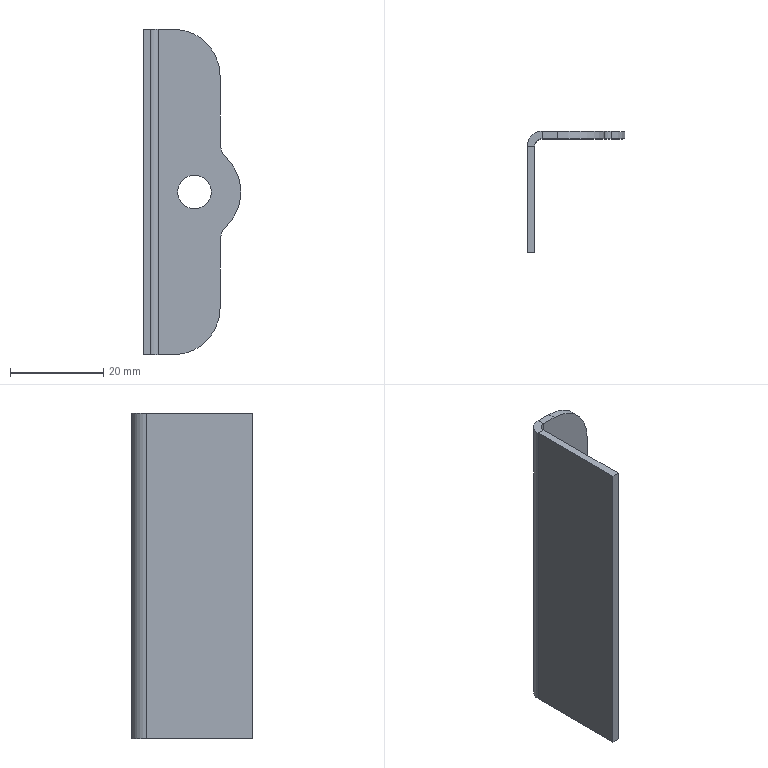Part | SolidWorks | features EdgeFlange 1, FlatPattern 1, SMBaseFlange 1, SheetMetal 1 | 1 solid | 22 faces | box 21 x 26 x 70 mm | volume 4418 mm3 | plane 13 | cylinder 9 | commonest cylinder face diameters 20 x3 7.2 x2 10 x2 3.2 x1 6.4 x1
STEP:
#1=CARTESIAN_POINT('',(2.75,-1.6,-3.6));
#2=VERTEX_POINT('',#1);
#3=CARTESIAN_POINT('',(2.75,-1.6,3.6));
#4=VERTEX_POINT('',#3);
#5=CARTESIAN_POINT('',(2.75,-1.6,0.));
#6=DIRECTION('',(0.,1.,0.));
#7=DIRECTION('',(0.,0.,1.));
#8=AXIS2_PLACEMENT_3D('',#5,#6,#7);
#9=CIRCLE('',#8,3.6);
#10=EDGE_CURVE('',#2,#4,#9,.T.);
#11=ORIENTED_EDGE('',*,*,#10,.F.);
#12=CARTESIAN_POINT('',(2.75,0.,-3.6));
#13=VERTEX_POINT('',#12);
#14=CARTESIAN_POINT('',(2.75,-1.6,-3.6));
#15=DIRECTION('',(0.,1.,0.));
#16=VECTOR('',#15,1000.);
#17=LINE('',#14,#16);
#18=EDGE_CURVE('',#2,#13,#17,.T.);
#19=ORIENTED_EDGE('',*,*,#18,.T.);
#20=CARTESIAN_POINT('',(2.75,0.,3.6));
#21=VERTEX_POINT('',#20);
#22=CARTESIAN_POINT('',(2.75,0.,0.));
#23=DIRECTION('',(0.,1.,0.));
#24=DIRECTION('',(0.,0.,1.));
#25=AXIS2_PLACEMENT_3D('',#22,#23,#24);
#26=CIRCLE('',#25,3.6);
#27=EDGE_CURVE('',#13,#21,#26,.T.);
#28=ORIENTED_EDGE('',*,*,#27,.T.);
#29=CARTESIAN_POINT('',(2.75,-1.6,3.6));
#30=DIRECTION('',(0.,1.,0.));
#31=VECTOR('',#30,1000.);
#32=LINE('',#29,#31);
#33=EDGE_CURVE('',#4,#21,#32,.T.);
#34=ORIENTED_EDGE('',*,*,#33,.F.);
#35=EDGE_LOOP('',(#11,#19,#28,#34));
#36=FACE_OUTER_BOUND('',#35,.T.);
#37=CARTESIAN_POINT('',(2.75,-1.6,0.));
#38=DIRECTION('',(0.,1.,0.));
#39=DIRECTION('',(0.,0.,1.));
#40=AXIS2_PLACEMENT_3D('',#37,#38,#39);
#41=CYLINDRICAL_SURFACE('',#40,3.6);
#42=ADVANCED_FACE('',(#36),#41,.F.);
#43=CARTESIAN_POINT('',(-1.75,-1.6,-35.));
#44=VERTEX_POINT('',#43);
#45=CARTESIAN_POINT('',(-5.05,-1.6,-35.));
#46=VERTEX_POINT('',#45);
#47=CARTESIAN_POINT('',(-8.25,-1.6,-35.));
#48=DIRECTION('',(-1.,0.,0.));
#49=VECTOR('',#48,1000.);
#50=LINE('',#47,#49);
#51=EDGE_CURVE('',#44,#46,#50,.T.);
#52=ORIENTED_EDGE('',*,*,#51,.T.);
#53=CARTESIAN_POINT('',(-5.05,0.,-35.));
#54=VERTEX_POINT('',#53);
#55=CARTESIAN_POINT('',(-5.05,-1.6,-35.));
#56=DIRECTION('',(0.,1.,0.));
#57=VECTOR('',#56,1000.);
#58=LINE('',#55,#57);
#59=EDGE_CURVE('',#46,#54,#58,.T.);
#60=ORIENTED_EDGE('',*,*,#59,.T.);
#61=CARTESIAN_POINT('',(-1.75,0.,-35.));
#62=VERTEX_POINT('',#61);
#63=CARTESIAN_POINT('',(-8.25,0.,-35.));
#64=DIRECTION('',(-1.,0.,0.));
#65=VECTOR('',#64,1000.);
#66=LINE('',#63,#65);
#67=EDGE_CURVE('',#62,#54,#66,.T.);
#68=ORIENTED_EDGE('',*,*,#67,.F.);
#69=CARTESIAN_POINT('',(-1.75,-1.6,-35.));
#70=DIRECTION('',(0.,1.,0.));
#71=VECTOR('',#70,1000.);
#72=LINE('',#69,#71);
#73=EDGE_CURVE('',#44,#62,#72,.T.);
#74=ORIENTED_EDGE('',*,*,#73,.F.);
#75=EDGE_LOOP('',(#52,#60,#68,#74));
#76=FACE_OUTER_BOUND('',#75,.T.);
#77=CARTESIAN_POINT('',(-8.25,-1.6,-35.));
#78=DIRECTION('',(0.,0.,-1.));
#79=DIRECTION('',(-1.,0.,0.));
#80=AXIS2_PLACEMENT_3D('',#77,#78,#79);
#81=PLANE('',#80);
#82=ADVANCED_FACE('',(#76),#81,.T.);
#83=CARTESIAN_POINT('',(2.75,-1.6,0.));
#84=DIRECTION('',(0.,1.,0.));
#85=DIRECTION('',(0.,0.,1.));
#86=AXIS2_PLACEMENT_3D('',#83,#84,#85);
#87=CIRCLE('',#86,3.6);
#88=EDGE_CURVE('',#4,#2,#87,.T.);
#89=ORIENTED_EDGE('',*,*,#88,.T.);
#90=ORIENTED_EDGE('',*,*,#10,.T.);
#91=EDGE_LOOP('',(#89,#90));
#92=FACE_BOUND('',#91,.T.);
#93=CARTESIAN_POINT('',(-5.05,-1.6,35.));
#94=VERTEX_POINT('',#93);
#95=CARTESIAN_POINT('',(-1.75,-1.6,35.));
#96=VERTEX_POINT('',#95);
#97=CARTESIAN_POINT('',(-8.25,-1.6,35.));
#98=DIRECTION('',(1.,0.,0.));
#99=VECTOR('',#98,1000.);
#100=LINE('',#97,#99);
#101=EDGE_CURVE('',#94,#96,#100,.T.);
#102=ORIENTED_EDGE('',*,*,#101,.F.);
#103=CARTESIAN_POINT('',(-5.05,-1.6,-35.));
#104=DIRECTION('',(0.,0.,1.));
#105=VECTOR('',#104,1000.);
#106=LINE('',#103,#105);
#107=EDGE_CURVE('',#46,#94,#106,.T.);
#108=ORIENTED_EDGE('',*,*,#107,.F.);
#109=ORIENTED_EDGE('',*,*,#51,.F.);
#110=CARTESIAN_POINT('',(8.25,-1.6,-25.));
#111=VERTEX_POINT('',#110);
#112=CARTESIAN_POINT('',(-1.75,-1.6,-25.));
#113=DIRECTION('',(0.,1.,0.));
#114=DIRECTION('',(0.,0.,1.));
#115=AXIS2_PLACEMENT_3D('',#112,#113,#114);
#116=CIRCLE('',#115,10.);
#117=EDGE_CURVE('',#111,#44,#116,.T.);
#118=ORIENTED_EDGE('',*,*,#117,.F.);
#119=CARTESIAN_POINT('',(8.25,-1.6,-10.712));
#120=VERTEX_POINT('',#119);
#121=CARTESIAN_POINT('',(8.25,-1.6,-25.));
#122=DIRECTION('',(0.,0.,-1.));
#123=VECTOR('',#122,1000.);
#124=LINE('',#121,#123);
#125=EDGE_CURVE('',#120,#111,#124,.T.);
#126=ORIENTED_EDGE('',*,*,#125,.F.);
#127=CARTESIAN_POINT('',(9.75,-1.6,-7.141));
#128=VERTEX_POINT('',#127);
#129=CARTESIAN_POINT('',(13.25,-1.6,-10.712));
#130=DIRECTION('',(0.,-1.,0.));
#131=DIRECTION('',(0.,0.,1.));
#132=AXIS2_PLACEMENT_3D('',#129,#130,#131);
#133=CIRCLE('',#132,5.);
#134=EDGE_CURVE('',#128,#120,#133,.T.);
#135=ORIENTED_EDGE('',*,*,#134,.F.);
#136=CARTESIAN_POINT('',(9.75,-1.6,7.141));
#137=VERTEX_POINT('',#136);
#138=CARTESIAN_POINT('',(2.75,-1.6,0.));
#139=DIRECTION('',(0.,1.,0.));
#140=DIRECTION('',(0.,0.,1.));
#141=AXIS2_PLACEMENT_3D('',#138,#139,#140);
#142=CIRCLE('',#141,10.);
#143=EDGE_CURVE('',#137,#128,#142,.T.);
#144=ORIENTED_EDGE('',*,*,#143,.F.);
#145=CARTESIAN_POINT('',(8.25,-1.6,10.712));
#146=VERTEX_POINT('',#145);
#147=CARTESIAN_POINT('',(13.25,-1.6,10.712));
#148=DIRECTION('',(0.,-1.,0.));
#149=DIRECTION('',(0.,0.,1.));
#150=AXIS2_PLACEMENT_3D('',#147,#148,#149);
#151=CIRCLE('',#150,5.);
#152=EDGE_CURVE('',#146,#137,#151,.T.);
#153=ORIENTED_EDGE('',*,*,#152,.F.);
#154=CARTESIAN_POINT('',(8.25,-1.6,25.));
#155=VERTEX_POINT('',#154);
#156=CARTESIAN_POINT('',(8.25,-1.6,10.712));
#157=DIRECTION('',(0.,0.,-1.));
#158=VECTOR('',#157,1000.);
#159=LINE('',#156,#158);
#160=EDGE_CURVE('',#155,#146,#159,.T.);
#161=ORIENTED_EDGE('',*,*,#160,.F.);
#162=CARTESIAN_POINT('',(-1.75,-1.6,25.));
#163=DIRECTION('',(0.,1.,0.));
#164=DIRECTION('',(0.,0.,-1.));
#165=AXIS2_PLACEMENT_3D('',#162,#163,#164);
#166=CIRCLE('',#165,10.);
#167=EDGE_CURVE('',#96,#155,#166,.T.);
#168=ORIENTED_EDGE('',*,*,#167,.F.);
#169=EDGE_LOOP('',(#102,#108,#109,#118,#126,#135,#144,#153,#161,#168));
#170=FACE_OUTER_BOUND('',#169,.T.);
#171=CARTESIAN_POINT('',(-1.75,-1.6,25.));
#172=DIRECTION('',(0.,-1.,0.));
#173=DIRECTION('',(0.,0.,-1.));
#174=AXIS2_PLACEMENT_3D('',#171,#172,#173);
#175=PLANE('',#174);
#176=ADVANCED_FACE('',(#92,#170),#175,.T.);
#177=CARTESIAN_POINT('',(2.75,0.,0.));
#178=DIRECTION('',(0.,1.,0.));
#179=DIRECTION('',(0.,0.,1.));
#180=AXIS2_PLACEMENT_3D('',#177,#178,#179);
#181=CIRCLE('',#180,3.6);
#182=EDGE_CURVE('',#21,#13,#181,.T.);
#183=ORIENTED_EDGE('',*,*,#182,.F.);
#184=ORIENTED_EDGE('',*,*,#27,.F.);
#185=EDGE_LOOP('',(#183,#184));
#186=FACE_BOUND('',#185,.T.);
#187=CARTESIAN_POINT('',(-5.05,0.,35.));
#188=VERTEX_POINT('',#187);
#189=CARTESIAN_POINT('',(-5.05,0.,-35.));
#190=DIRECTION('',(0.,0.,1.));
#191=VECTOR('',#190,1000.);
#192=LINE('',#189,#191);
#193=EDGE_CURVE('',#54,#188,#192,.T.);
#194=ORIENTED_EDGE('',*,*,#193,.T.);
#195=CARTESIAN_POINT('',(-1.75,0.,35.));
#196=VERTEX_POINT('',#195);
#197=CARTESIAN_POINT('',(-8.25,0.,35.));
#198=DIRECTION('',(1.,0.,0.));
#199=VECTOR('',#198,1000.);
#200=LINE('',#197,#199);
#201=EDGE_CURVE('',#188,#196,#200,.T.);
#202=ORIENTED_EDGE('',*,*,#201,.T.);
#203=CARTESIAN_POINT('',(8.25,0.,25.));
#204=VERTEX_POINT('',#203);
#205=CARTESIAN_POINT('',(-1.75,0.,25.));
#206=DIRECTION('',(0.,1.,0.));
#207=DIRECTION('',(0.,0.,-1.));
#208=AXIS2_PLACEMENT_3D('',#205,#206,#207);
#209=CIRCLE('',#208,10.);
#210=EDGE_CURVE('',#196,#204,#209,.T.);
#211=ORIENTED_EDGE('',*,*,#210,.T.);
#212=CARTESIAN_POINT('',(8.25,0.,10.712));
#213=VERTEX_POINT('',#212);
#214=CARTESIAN_POINT('',(8.25,0.,10.712));
#215=DIRECTION('',(0.,0.,-1.));
#216=VECTOR('',#215,1000.);
#217=LINE('',#214,#216);
#218=EDGE_CURVE('',#204,#213,#217,.T.);
#219=ORIENTED_EDGE('',*,*,#218,.T.);
#220=CARTESIAN_POINT('',(9.75,0.,7.141));
#221=VERTEX_POINT('',#220);
#222=CARTESIAN_POINT('',(13.25,0.,10.712));
#223=DIRECTION('',(0.,-1.,0.));
#224=DIRECTION('',(0.,0.,1.));
#225=AXIS2_PLACEMENT_3D('',#222,#223,#224);
#226=CIRCLE('',#225,5.);
#227=EDGE_CURVE('',#213,#221,#226,.T.);
#228=ORIENTED_EDGE('',*,*,#227,.T.);
#229=CARTESIAN_POINT('',(9.75,0.,-7.141));
#230=VERTEX_POINT('',#229);
#231=CARTESIAN_POINT('',(2.75,0.,0.));
#232=DIRECTION('',(0.,1.,0.));
#233=DIRECTION('',(0.,0.,1.));
#234=AXIS2_PLACEMENT_3D('',#231,#232,#233);
#235=CIRCLE('',#234,10.);
#236=EDGE_CURVE('',#221,#230,#235,.T.);
#237=ORIENTED_EDGE('',*,*,#236,.T.);
#238=CARTESIAN_POINT('',(8.25,0.,-10.712));
#239=VERTEX_POINT('',#238);
#240=CARTESIAN_POINT('',(13.25,0.,-10.712));
#241=DIRECTION('',(0.,-1.,0.));
#242=DIRECTION('',(0.,0.,1.));
#243=AXIS2_PLACEMENT_3D('',#240,#241,#242);
#244=CIRCLE('',#243,5.);
#245=EDGE_CURVE('',#230,#239,#244,.T.);
#246=ORIENTED_EDGE('',*,*,#245,.T.);
#247=CARTESIAN_POINT('',(8.25,0.,-25.));
#248=VERTEX_POINT('',#247);
#249=CARTESIAN_POINT('',(8.25,0.,-25.));
#250=DIRECTION('',(0.,0.,-1.));
#251=VECTOR('',#250,1000.);
#252=LINE('',#249,#251);
#253=EDGE_CURVE('',#239,#248,#252,.T.);
#254=ORIENTED_EDGE('',*,*,#253,.T.);
#255=CARTESIAN_POINT('',(-1.75,0.,-25.));
#256=DIRECTION('',(0.,1.,0.));
#257=DIRECTION('',(0.,0.,1.));
#258=AXIS2_PLACEMENT_3D('',#255,#256,#257);
#259=CIRCLE('',#258,10.);
#260=EDGE_CURVE('',#248,#62,#259,.T.);
#261=ORIENTED_EDGE('',*,*,#260,.T.);
#262=ORIENTED_EDGE('',*,*,#67,.T.);
#263=EDGE_LOOP('',(#194,#202,#211,#219,#228,#237,#246,#254,#261,#262));
#264=FACE_OUTER_BOUND('',#263,.T.);
#265=CARTESIAN_POINT('',(-1.75,0.,25.));
#266=DIRECTION('',(0.,-1.,0.));
#267=DIRECTION('',(0.,0.,-1.));
#268=AXIS2_PLACEMENT_3D('',#265,#266,#267);
#269=PLANE('',#268);
#270=ADVANCED_FACE('',(#186,#264),#269,.F.);
#271=ORIENTED_EDGE('',*,*,#260,.F.);
#272=CARTESIAN_POINT('',(8.25,-1.6,-25.));
#273=DIRECTION('',(0.,1.,0.));
#274=VECTOR('',#273,1000.);
#275=LINE('',#272,#274);
#276=EDGE_CURVE('',#111,#248,#275,.T.);
#277=ORIENTED_EDGE('',*,*,#276,.F.);
#278=ORIENTED_EDGE('',*,*,#117,.T.);
#279=ORIENTED_EDGE('',*,*,#73,.T.);
#280=EDGE_LOOP('',(#271,#277,#278,#279));
#281=FACE_OUTER_BOUND('',#280,.T.);
#282=CARTESIAN_POINT('',(-1.75,-1.6,-25.));
#283=DIRECTION('',(0.,1.,0.));
#284=DIRECTION('',(0.,0.,1.));
#285=AXIS2_PLACEMENT_3D('',#282,#283,#284);
#286=CYLINDRICAL_SURFACE('',#285,10.);
#287=ADVANCED_FACE('',(#281),#286,.T.);
#288=ORIENTED_EDGE('',*,*,#253,.F.);
#289=CARTESIAN_POINT('',(8.25,-1.6,-10.712));
#290=DIRECTION('',(0.,1.,0.));
#291=VECTOR('',#290,1000.);
#292=LINE('',#289,#291);
#293=EDGE_CURVE('',#120,#239,#292,.T.);
#294=ORIENTED_EDGE('',*,*,#293,.F.);
#295=ORIENTED_EDGE('',*,*,#125,.T.);
#296=ORIENTED_EDGE('',*,*,#276,.T.);
#297=EDGE_LOOP('',(#288,#294,#295,#296));
#298=FACE_OUTER_BOUND('',#297,.T.);
#299=CARTESIAN_POINT('',(8.25,-1.6,-25.));
#300=DIRECTION('',(1.,0.,0.));
#301=DIRECTION('',(0.,0.,-1.));
#302=AXIS2_PLACEMENT_3D('',#299,#300,#301);
#303=PLANE('',#302);
#304=ADVANCED_FACE('',(#298),#303,.T.);
#305=ORIENTED_EDGE('',*,*,#245,.F.);
#306=CARTESIAN_POINT('',(9.75,-1.6,-7.141));
#307=DIRECTION('',(0.,1.,0.));
#308=VECTOR('',#307,1000.);
#309=LINE('',#306,#308);
#310=EDGE_CURVE('',#128,#230,#309,.T.);
#311=ORIENTED_EDGE('',*,*,#310,.F.);
#312=ORIENTED_EDGE('',*,*,#134,.T.);
#313=ORIENTED_EDGE('',*,*,#293,.T.);
#314=EDGE_LOOP('',(#305,#311,#312,#313));
#315=FACE_OUTER_BOUND('',#314,.T.);
#316=CARTESIAN_POINT('',(13.25,-1.6,-10.712));
#317=DIRECTION('',(0.,1.,0.));
#318=DIRECTION('',(0.,0.,1.));
#319=AXIS2_PLACEMENT_3D('',#316,#317,#318);
#320=CYLINDRICAL_SURFACE('',#319,5.);
#321=ADVANCED_FACE('',(#315),#320,.F.);
#322=ORIENTED_EDGE('',*,*,#236,.F.);
#323=CARTESIAN_POINT('',(9.75,-1.6,7.141));
#324=DIRECTION('',(0.,1.,0.));
#325=VECTOR('',#324,1000.);
#326=LINE('',#323,#325);
#327=EDGE_CURVE('',#137,#221,#326,.T.);
#328=ORIENTED_EDGE('',*,*,#327,.F.);
#329=ORIENTED_EDGE('',*,*,#143,.T.);
#330=ORIENTED_EDGE('',*,*,#310,.T.);
#331=EDGE_LOOP('',(#322,#328,#329,#330));
#332=FACE_OUTER_BOUND('',#331,.T.);
#333=CARTESIAN_POINT('',(2.75,-1.6,0.));
#334=DIRECTION('',(0.,1.,0.));
#335=DIRECTION('',(0.,0.,1.));
#336=AXIS2_PLACEMENT_3D('',#333,#334,#335);
#337=CYLINDRICAL_SURFACE('',#336,10.);
#338=ADVANCED_FACE('',(#332),#337,.T.);
#339=ORIENTED_EDGE('',*,*,#227,.F.);
#340=CARTESIAN_POINT('',(8.25,-1.6,10.712));
#341=DIRECTION('',(0.,1.,0.));
#342=VECTOR('',#341,1000.);
#343=LINE('',#340,#342);
#344=EDGE_CURVE('',#146,#213,#343,.T.);
#345=ORIENTED_EDGE('',*,*,#344,.F.);
#346=ORIENTED_EDGE('',*,*,#152,.T.);
#347=ORIENTED_EDGE('',*,*,#327,.T.);
#348=EDGE_LOOP('',(#339,#345,#346,#347));
#349=FACE_OUTER_BOUND('',#348,.T.);
#350=CARTESIAN_POINT('',(13.25,-1.6,10.712));
#351=DIRECTION('',(0.,1.,0.));
#352=DIRECTION('',(0.,0.,1.));
#353=AXIS2_PLACEMENT_3D('',#350,#351,#352);
#354=CYLINDRICAL_SURFACE('',#353,5.);
#355=ADVANCED_FACE('',(#349),#354,.F.);
#356=ORIENTED_EDGE('',*,*,#218,.F.);
#357=CARTESIAN_POINT('',(8.25,-1.6,25.));
#358=DIRECTION('',(0.,1.,0.));
#359=VECTOR('',#358,1000.);
#360=LINE('',#357,#359);
#361=EDGE_CURVE('',#155,#204,#360,.T.);
#362=ORIENTED_EDGE('',*,*,#361,.F.);
#363=ORIENTED_EDGE('',*,*,#160,.T.);
#364=ORIENTED_EDGE('',*,*,#344,.T.);
#365=EDGE_LOOP('',(#356,#362,#363,#364));
#366=FACE_OUTER_BOUND('',#365,.T.);
#367=CARTESIAN_POINT('',(8.25,-1.6,10.712));
#368=DIRECTION('',(1.,0.,0.));
#369=DIRECTION('',(0.,0.,-1.));
#370=AXIS2_PLACEMENT_3D('',#367,#368,#369);
#371=PLANE('',#370);
#372=ADVANCED_FACE('',(#366),#371,.T.);
#373=ORIENTED_EDGE('',*,*,#210,.F.);
#374=CARTESIAN_POINT('',(-1.75,-1.6,35.));
#375=DIRECTION('',(0.,1.,0.));
#376=VECTOR('',#375,1000.);
#377=LINE('',#374,#376);
#378=EDGE_CURVE('',#96,#196,#377,.T.);
#379=ORIENTED_EDGE('',*,*,#378,.F.);
#380=ORIENTED_EDGE('',*,*,#167,.T.);
#381=ORIENTED_EDGE('',*,*,#361,.T.);
#382=EDGE_LOOP('',(#373,#379,#380,#381));
#383=FACE_OUTER_BOUND('',#382,.T.);
#384=CARTESIAN_POINT('',(-1.75,-1.6,25.));
#385=DIRECTION('',(0.,1.,0.));
#386=DIRECTION('',(0.,0.,1.));
#387=AXIS2_PLACEMENT_3D('',#384,#385,#386);
#388=CYLINDRICAL_SURFACE('',#387,10.);
#389=ADVANCED_FACE('',(#383),#388,.T.);
#390=CARTESIAN_POINT('',(-5.05,-1.6,35.));
#391=DIRECTION('',(0.,1.,0.));
#392=VECTOR('',#391,1000.);
#393=LINE('',#390,#392);
#394=EDGE_CURVE('',#94,#188,#393,.T.);
#395=ORIENTED_EDGE('',*,*,#394,.F.);
#396=ORIENTED_EDGE('',*,*,#101,.T.);
#397=ORIENTED_EDGE('',*,*,#378,.T.);
#398=ORIENTED_EDGE('',*,*,#201,.F.);
#399=EDGE_LOOP('',(#395,#396,#397,#398));
#400=FACE_OUTER_BOUND('',#399,.T.);
#401=CARTESIAN_POINT('',(-8.25,-1.6,35.));
#402=DIRECTION('',(0.,0.,1.));
#403=DIRECTION('',(1.,0.,0.));
#404=AXIS2_PLACEMENT_3D('',#401,#402,#403);
#405=PLANE('',#404);
#406=ADVANCED_FACE('',(#400),#405,.T.);
#407=ORIENTED_EDGE('',*,*,#18,.F.);
#408=ORIENTED_EDGE('',*,*,#88,.F.);
#409=ORIENTED_EDGE('',*,*,#33,.T.);
#410=ORIENTED_EDGE('',*,*,#182,.T.);
#411=EDGE_LOOP('',(#407,#408,#409,#410));
#412=FACE_OUTER_BOUND('',#411,.T.);
#413=CARTESIAN_POINT('',(2.75,-1.6,0.));
#414=DIRECTION('',(0.,1.,0.));
#415=DIRECTION('',(0.,0.,1.));
#416=AXIS2_PLACEMENT_3D('',#413,#414,#415);
#417=CYLINDRICAL_SURFACE('',#416,3.6);
#418=ADVANCED_FACE('',(#412),#417,.F.);
#419=CARTESIAN_POINT('',(-6.65,-3.2,35.));
#420=VERTEX_POINT('',#419);
#421=CARTESIAN_POINT('',(-8.25,-3.2,35.));
#422=VERTEX_POINT('',#421);
#423=CARTESIAN_POINT('',(-8.25,-3.2,35.));
#424=DIRECTION('',(-1.,0.,0.));
#425=VECTOR('',#424,1000.);
#426=LINE('',#423,#425);
#427=EDGE_CURVE('',#420,#422,#426,.T.);
#428=ORIENTED_EDGE('',*,*,#427,.F.);
#429=CARTESIAN_POINT('',(-5.05,-3.2,35.));
#430=DIRECTION('',(0.,0.,1.));
#431=DIRECTION('',(-1.,0.,0.));
#432=AXIS2_PLACEMENT_3D('',#429,#430,#431);
#433=CIRCLE('',#432,1.6);
#434=EDGE_CURVE('',#94,#420,#433,.T.);
#435=ORIENTED_EDGE('',*,*,#434,.F.);
#436=ORIENTED_EDGE('',*,*,#394,.T.);
#437=CARTESIAN_POINT('',(-5.05,-3.2,35.));
#438=DIRECTION('',(0.,0.,1.));
#439=DIRECTION('',(-1.,0.,0.));
#440=AXIS2_PLACEMENT_3D('',#437,#438,#439);
#441=CIRCLE('',#440,3.2);
#442=EDGE_CURVE('',#188,#422,#441,.T.);
#443=ORIENTED_EDGE('',*,*,#442,.T.);
#444=EDGE_LOOP('',(#428,#435,#436,#443));
#445=FACE_OUTER_BOUND('',#444,.T.);
#446=CARTESIAN_POINT('',(-5.05,-3.2,35.));
#447=DIRECTION('',(0.,0.,1.));
#448=DIRECTION('',(1.,0.,0.));
#449=AXIS2_PLACEMENT_3D('',#446,#447,#448);
#450=PLANE('',#449);
#451=ADVANCED_FACE('',(#445),#450,.T.);
#452=CARTESIAN_POINT('',(-6.65,-3.2,-35.));
#453=VERTEX_POINT('',#452);
#454=CARTESIAN_POINT('',(-5.05,-3.2,-35.));
#455=DIRECTION('',(0.,0.,-1.));
#456=DIRECTION('',(-1.,0.,0.));
#457=AXIS2_PLACEMENT_3D('',#454,#455,#456);
#458=CIRCLE('',#457,1.6);
#459=EDGE_CURVE('',#453,#46,#458,.T.);
#460=ORIENTED_EDGE('',*,*,#459,.F.);
#461=CARTESIAN_POINT('',(-8.25,-3.2,-35.));
#462=VERTEX_POINT('',#461);
#463=CARTESIAN_POINT('',(-6.65,-3.2,-35.));
#464=DIRECTION('',(-1.,0.,0.));
#465=VECTOR('',#464,1000.);
#466=LINE('',#463,#465);
#467=EDGE_CURVE('',#453,#462,#466,.T.);
#468=ORIENTED_EDGE('',*,*,#467,.T.);
#469=CARTESIAN_POINT('',(-5.05,-3.2,-35.));
#470=DIRECTION('',(0.,0.,-1.));
#471=DIRECTION('',(-1.,0.,0.));
#472=AXIS2_PLACEMENT_3D('',#469,#470,#471);
#473=CIRCLE('',#472,3.2);
#474=EDGE_CURVE('',#462,#54,#473,.T.);
#475=ORIENTED_EDGE('',*,*,#474,.T.);
#476=ORIENTED_EDGE('',*,*,#59,.F.);
#477=EDGE_LOOP('',(#460,#468,#475,#476));
#478=FACE_OUTER_BOUND('',#477,.T.);
#479=CARTESIAN_POINT('',(-5.05,-3.2,-35.));
#480=DIRECTION('',(0.,0.,1.));
#481=DIRECTION('',(1.,0.,0.));
#482=AXIS2_PLACEMENT_3D('',#479,#480,#481);
#483=PLANE('',#482);
#484=ADVANCED_FACE('',(#478),#483,.F.);
#485=ORIENTED_EDGE('',*,*,#193,.F.);
#486=ORIENTED_EDGE('',*,*,#474,.F.);
#487=CARTESIAN_POINT('',(-8.25,-3.2,35.));
#488=DIRECTION('',(0.,0.,1.));
#489=VECTOR('',#488,1000.);
#490=LINE('',#487,#489);
#491=EDGE_CURVE('',#462,#422,#490,.T.);
#492=ORIENTED_EDGE('',*,*,#491,.T.);
#493=ORIENTED_EDGE('',*,*,#442,.F.);
#494=EDGE_LOOP('',(#485,#486,#492,#493));
#495=FACE_OUTER_BOUND('',#494,.T.);
#496=CARTESIAN_POINT('',(-5.05,-3.2,-35.));
#497=DIRECTION('',(0.,0.,-1.));
#498=DIRECTION('',(-1.,0.,0.));
#499=AXIS2_PLACEMENT_3D('',#496,#497,#498);
#500=CYLINDRICAL_SURFACE('',#499,3.2);
#501=ADVANCED_FACE('',(#495),#500,.T.);
#502=ORIENTED_EDGE('',*,*,#107,.T.);
#503=ORIENTED_EDGE('',*,*,#434,.T.);
#504=CARTESIAN_POINT('',(-6.65,-3.2,35.));
#505=DIRECTION('',(0.,0.,-1.));
#506=VECTOR('',#505,1000.);
#507=LINE('',#504,#506);
#508=EDGE_CURVE('',#420,#453,#507,.T.);
#509=ORIENTED_EDGE('',*,*,#508,.T.);
#510=ORIENTED_EDGE('',*,*,#459,.T.);
#511=EDGE_LOOP('',(#502,#503,#509,#510));
#512=FACE_OUTER_BOUND('',#511,.T.);
#513=CARTESIAN_POINT('',(-5.05,-3.2,-35.));
#514=DIRECTION('',(0.,0.,-1.));
#515=DIRECTION('',(-1.,0.,0.));
#516=AXIS2_PLACEMENT_3D('',#513,#514,#515);
#517=CYLINDRICAL_SURFACE('',#516,1.6);
#518=ADVANCED_FACE('',(#512),#517,.F.);
#519=ORIENTED_EDGE('',*,*,#467,.F.);
#520=CARTESIAN_POINT('',(-6.65,-26.,-35.));
#521=VERTEX_POINT('',#520);
#522=CARTESIAN_POINT('',(-6.65,-26.,-35.));
#523=DIRECTION('',(0.,-1.,0.));
#524=VECTOR('',#523,1000.);
#525=LINE('',#522,#524);
#526=EDGE_CURVE('',#453,#521,#525,.T.);
#527=ORIENTED_EDGE('',*,*,#526,.T.);
#528=CARTESIAN_POINT('',(-8.25,-26.,-35.));
#529=VERTEX_POINT('',#528);
#530=CARTESIAN_POINT('',(-8.25,-26.,-35.));
#531=DIRECTION('',(1.,0.,0.));
#532=VECTOR('',#531,1000.);
#533=LINE('',#530,#532);
#534=EDGE_CURVE('',#529,#521,#533,.T.);
#535=ORIENTED_EDGE('',*,*,#534,.F.);
#536=CARTESIAN_POINT('',(-8.25,0.,-35.));
#537=DIRECTION('',(0.,-1.,0.));
#538=VECTOR('',#537,1000.);
#539=LINE('',#536,#538);
#540=EDGE_CURVE('',#462,#529,#539,.T.);
#541=ORIENTED_EDGE('',*,*,#540,.F.);
#542=EDGE_LOOP('',(#519,#527,#535,#541));
#543=FACE_OUTER_BOUND('',#542,.T.);
#544=CARTESIAN_POINT('',(-8.25,-26.,-35.));
#545=DIRECTION('',(0.,0.,1.));
#546=DIRECTION('',(1.,0.,0.));
#547=AXIS2_PLACEMENT_3D('',#544,#545,#546);
#548=PLANE('',#547);
#549=ADVANCED_FACE('',(#543),#548,.F.);
#550=ORIENTED_EDGE('',*,*,#427,.T.);
#551=CARTESIAN_POINT('',(-8.25,-26.,35.));
#552=VERTEX_POINT('',#551);
#553=CARTESIAN_POINT('',(-8.25,0.,35.));
#554=DIRECTION('',(0.,1.,0.));
#555=VECTOR('',#554,1000.);
#556=LINE('',#553,#555);
#557=EDGE_CURVE('',#552,#422,#556,.T.);
#558=ORIENTED_EDGE('',*,*,#557,.F.);
#559=CARTESIAN_POINT('',(-6.65,-26.,35.));
#560=VERTEX_POINT('',#559);
#561=CARTESIAN_POINT('',(-8.25,-26.,35.));
#562=DIRECTION('',(1.,0.,0.));
#563=VECTOR('',#562,1000.);
#564=LINE('',#561,#563);
#565=EDGE_CURVE('',#552,#560,#564,.T.);
#566=ORIENTED_EDGE('',*,*,#565,.T.);
#567=CARTESIAN_POINT('',(-6.65,-1.6,35.));
#568=DIRECTION('',(0.,1.,0.));
#569=VECTOR('',#568,1000.);
#570=LINE('',#567,#569);
#571=EDGE_CURVE('',#560,#420,#570,.T.);
#572=ORIENTED_EDGE('',*,*,#571,.T.);
#573=EDGE_LOOP('',(#550,#558,#566,#572));
#574=FACE_OUTER_BOUND('',#573,.T.);
#575=CARTESIAN_POINT('',(-8.25,-1.6,35.));
#576=DIRECTION('',(0.,0.,-1.));
#577=DIRECTION('',(-1.,0.,0.));
#578=AXIS2_PLACEMENT_3D('',#575,#576,#577);
#579=PLANE('',#578);
#580=ADVANCED_FACE('',(#574),#579,.F.);
#581=ORIENTED_EDGE('',*,*,#491,.F.);
#582=ORIENTED_EDGE('',*,*,#540,.T.);
#583=CARTESIAN_POINT('',(-8.25,-26.,0.));
#584=DIRECTION('',(0.,0.,1.));
#585=VECTOR('',#584,1000.);
#586=LINE('',#583,#585);
#587=EDGE_CURVE('',#529,#552,#586,.T.);
#588=ORIENTED_EDGE('',*,*,#587,.T.);
#589=ORIENTED_EDGE('',*,*,#557,.T.);
#590=EDGE_LOOP('',(#581,#582,#588,#589));
#591=FACE_OUTER_BOUND('',#590,.T.);
#592=CARTESIAN_POINT('',(-8.25,0.,0.));
#593=DIRECTION('',(1.,0.,0.));
#594=DIRECTION('',(0.,1.,0.));
#595=AXIS2_PLACEMENT_3D('',#592,#593,#594);
#596=PLANE('',#595);
#597=ADVANCED_FACE('',(#591),#596,.F.);
#598=ORIENTED_EDGE('',*,*,#526,.F.);
#599=ORIENTED_EDGE('',*,*,#508,.F.);
#600=ORIENTED_EDGE('',*,*,#571,.F.);
#601=CARTESIAN_POINT('',(-6.65,-26.,35.));
#602=DIRECTION('',(0.,0.,1.));
#603=VECTOR('',#602,1000.);
#604=LINE('',#601,#603);
#605=EDGE_CURVE('',#521,#560,#604,.T.);
#606=ORIENTED_EDGE('',*,*,#605,.F.);
#607=EDGE_LOOP('',(#598,#599,#600,#606));
#608=FACE_OUTER_BOUND('',#607,.T.);
#609=CARTESIAN_POINT('',(-6.65,0.,0.));
#610=DIRECTION('',(1.,0.,0.));
#611=DIRECTION('',(0.,1.,0.));
#612=AXIS2_PLACEMENT_3D('',#609,#610,#611);
#613=PLANE('',#612);
#614=ADVANCED_FACE('',(#608),#613,.T.);
#615=ORIENTED_EDGE('',*,*,#605,.T.);
#616=ORIENTED_EDGE('',*,*,#565,.F.);
#617=ORIENTED_EDGE('',*,*,#587,.F.);
#618=ORIENTED_EDGE('',*,*,#534,.T.);
#619=EDGE_LOOP('',(#615,#616,#617,#618));
#620=FACE_OUTER_BOUND('',#619,.T.);
#621=CARTESIAN_POINT('',(-8.25,-26.,35.));
#622=DIRECTION('',(0.,1.,0.));
#623=DIRECTION('',(-1.,0.,0.));
#624=AXIS2_PLACEMENT_3D('',#621,#622,#623);
#625=PLANE('',#624);
#626=ADVANCED_FACE('',(#620),#625,.F.);
#627=CLOSED_SHELL('',(#42,#82,#176,#270,#287,#304,#321,#338,#355,#372,#389,#406,#418,#451,#484,#501,#518,#549,#580,#597,#614,#626));
#628=MANIFOLD_SOLID_BREP('',#627);
#629=CARTESIAN_POINT('',(0.,0.,0.));
#630=DIRECTION('',(0.,0.,1.));
#631=DIRECTION('',(1.,0.,0.));
#632=AXIS2_PLACEMENT_3D('',#629,#630,#631);
#633=(LENGTH_UNIT()NAMED_UNIT(*)SI_UNIT(.MILLI.,.METRE.));
#634=UNCERTAINTY_MEASURE_WITH_UNIT(LENGTH_MEASURE(0.00001),#633,'','');
#635=(NAMED_UNIT(*)PLANE_ANGLE_UNIT()SI_UNIT($,.RADIAN.));
#636=(NAMED_UNIT(*)SI_UNIT($,.STERADIAN.)SOLID_ANGLE_UNIT());
#637=(GEOMETRIC_REPRESENTATION_CONTEXT(3)GLOBAL_UNCERTAINTY_ASSIGNED_CONTEXT((#634))GLOBAL_UNIT_ASSIGNED_CONTEXT((#633,#635,#636))REPRESENTATION_CONTEXT('',''));
#638=ADVANCED_BREP_SHAPE_REPRESENTATION('',(#628,#632),#637);